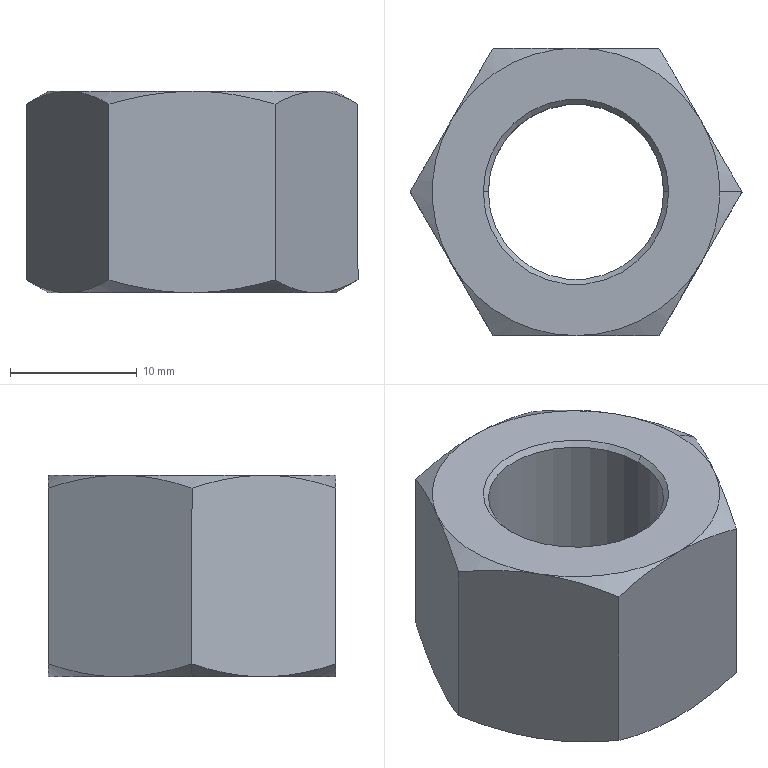Part | SolidWorks | features Cut 2, Chamfer 1, Extrusion 1 | 1 solid | 28 faces | box 26.2 x 22.69 x 15.9 mm | volume 4666 mm3 | cone 18 | plane 8 | cylinder 2 | commonest cylinder face diameters 13.835 x2
STEP:
#1=CARTESIAN_POINT('',(-6.918,0.,15.503));
#2=VERTEX_POINT('',#1);
#3=CARTESIAN_POINT('',(6.918,0.,15.503));
#4=VERTEX_POINT('',#3);
#5=CARTESIAN_POINT('',(0.,0.,15.503));
#6=DIRECTION('',(0.,0.,1.));
#7=DIRECTION('',(-1.,0.,0.));
#8=AXIS2_PLACEMENT_3D('',#5,#6,#7);
#9=CIRCLE('',#8,6.918);
#10=EDGE_CURVE('',#2,#4,#9,.T.);
#11=ORIENTED_EDGE('',*,*,#10,.F.);
#12=CARTESIAN_POINT('',(-7.315,0.,15.9));
#13=VERTEX_POINT('',#12);
#14=CARTESIAN_POINT('',(-6.918,0.,15.503));
#15=DIRECTION('',(-0.7071,0.,0.7071));
#16=VECTOR('',#15,1000.);
#17=LINE('',#14,#16);
#18=EDGE_CURVE('',#2,#13,#17,.T.);
#19=ORIENTED_EDGE('',*,*,#18,.T.);
#20=CARTESIAN_POINT('',(7.315,0.,15.9));
#21=VERTEX_POINT('',#20);
#22=CARTESIAN_POINT('',(0.,0.,15.9));
#23=DIRECTION('',(0.,0.,-1.));
#24=DIRECTION('',(-1.,0.,0.));
#25=AXIS2_PLACEMENT_3D('',#22,#23,#24);
#26=CIRCLE('',#25,7.315);
#27=EDGE_CURVE('',#21,#13,#26,.T.);
#28=ORIENTED_EDGE('',*,*,#27,.F.);
#29=CARTESIAN_POINT('',(6.918,0.,15.503));
#30=DIRECTION('',(0.7071,0.,0.7071));
#31=VECTOR('',#30,1000.);
#32=LINE('',#29,#31);
#33=EDGE_CURVE('',#4,#21,#32,.T.);
#34=ORIENTED_EDGE('',*,*,#33,.F.);
#35=EDGE_LOOP('',(#11,#19,#28,#34));
#36=FACE_OUTER_BOUND('',#35,.T.);
#37=CARTESIAN_POINT('',(0.,0.,15.503));
#38=DIRECTION('',(0.,0.,1.));
#39=DIRECTION('',(1.,0.,0.));
#40=AXIS2_PLACEMENT_3D('',#37,#38,#39);
#41=CONICAL_SURFACE('',#40,6.918,0.7854);
#42=ADVANCED_FACE('',(#36),#41,.F.);
#43=CARTESIAN_POINT('',(6.918,0.,0.3975));
#44=VERTEX_POINT('',#43);
#45=CARTESIAN_POINT('',(-6.918,0.,0.3975));
#46=VERTEX_POINT('',#45);
#47=CARTESIAN_POINT('',(0.,0.,0.3975));
#48=DIRECTION('',(0.,0.,-1.));
#49=DIRECTION('',(-1.,0.,0.));
#50=AXIS2_PLACEMENT_3D('',#47,#48,#49);
#51=CIRCLE('',#50,6.918);
#52=EDGE_CURVE('',#44,#46,#51,.T.);
#53=ORIENTED_EDGE('',*,*,#52,.F.);
#54=CARTESIAN_POINT('',(7.315,0.,0.));
#55=VERTEX_POINT('',#54);
#56=CARTESIAN_POINT('',(7.315,0.,0.));
#57=DIRECTION('',(0.7071,0.,-0.7071));
#58=VECTOR('',#57,1000.);
#59=LINE('',#56,#58);
#60=EDGE_CURVE('',#44,#55,#59,.T.);
#61=ORIENTED_EDGE('',*,*,#60,.T.);
#62=CARTESIAN_POINT('',(-7.315,0.,0.));
#63=VERTEX_POINT('',#62);
#64=CARTESIAN_POINT('',(0.,0.,0.));
#65=DIRECTION('',(0.,0.,1.));
#66=DIRECTION('',(-1.,0.,0.));
#67=AXIS2_PLACEMENT_3D('',#64,#65,#66);
#68=CIRCLE('',#67,7.315);
#69=EDGE_CURVE('',#63,#55,#68,.T.);
#70=ORIENTED_EDGE('',*,*,#69,.F.);
#71=CARTESIAN_POINT('',(-7.315,0.,0.));
#72=DIRECTION('',(-0.7071,0.,-0.7071));
#73=VECTOR('',#72,1000.);
#74=LINE('',#71,#73);
#75=EDGE_CURVE('',#46,#63,#74,.T.);
#76=ORIENTED_EDGE('',*,*,#75,.F.);
#77=EDGE_LOOP('',(#53,#61,#70,#76));
#78=FACE_OUTER_BOUND('',#77,.T.);
#79=CARTESIAN_POINT('',(0.,0.,0.));
#80=DIRECTION('',(0.,0.,-1.));
#81=DIRECTION('',(-1.,0.,0.));
#82=AXIS2_PLACEMENT_3D('',#79,#80,#81);
#83=CONICAL_SURFACE('',#82,7.315,0.7854);
#84=ADVANCED_FACE('',(#78),#83,.F.);
#85=CARTESIAN_POINT('',(9.825,5.672,15.9));
#86=VERTEX_POINT('',#85);
#87=CARTESIAN_POINT('',(11.345,0.,15.9));
#88=VERTEX_POINT('',#87);
#89=CARTESIAN_POINT('',(0.,0.,15.9));
#90=DIRECTION('',(0.,0.,-1.));
#91=DIRECTION('',(-1.,0.,0.));
#92=AXIS2_PLACEMENT_3D('',#89,#90,#91);
#93=CIRCLE('',#92,11.345);
#94=EDGE_CURVE('',#86,#88,#93,.T.);
#95=ORIENTED_EDGE('',*,*,#94,.T.);
#96=CARTESIAN_POINT('',(13.1,0.,14.887));
#97=VERTEX_POINT('',#96);
#98=CARTESIAN_POINT('',(11.345,0.,15.9));
#99=DIRECTION('',(0.866,0.,-0.5));
#100=VECTOR('',#99,1000.);
#101=LINE('',#98,#100);
#102=EDGE_CURVE('',#88,#97,#101,.T.);
#103=ORIENTED_EDGE('',*,*,#102,.T.);
#104=CARTESIAN_POINT('',(13.1,0.,14.887));
#105=CARTESIAN_POINT('',(12.564,0.9279,15.196));
#106=CARTESIAN_POINT('',(12.025,1.863,15.451));
#107=CARTESIAN_POINT('',(10.934,3.752,15.803));
#108=CARTESIAN_POINT('',(10.383,4.706,15.9));
#109=CARTESIAN_POINT('',(9.825,5.672,15.9));
#110=B_SPLINE_CURVE_WITH_KNOTS('',3,(#104,#105,#106,#107,#108,#109),.UNSPECIFIED.,.F.,.F.,(4,2,4),(0.000000238,0.003314,0.006628),.UNSPECIFIED.);
#111=EDGE_CURVE('',#97,#86,#110,.T.);
#112=ORIENTED_EDGE('',*,*,#111,.T.);
#113=EDGE_LOOP('',(#95,#103,#112));
#114=FACE_OUTER_BOUND('',#113,.T.);
#115=CARTESIAN_POINT('',(0.,0.,15.9));
#116=DIRECTION('',(0.,0.,-1.));
#117=DIRECTION('',(1.,0.,0.));
#118=AXIS2_PLACEMENT_3D('',#115,#116,#117);
#119=CONICAL_SURFACE('',#118,11.345,1.047);
#120=ADVANCED_FACE('',(#114),#119,.T.);
#121=CARTESIAN_POINT('',(-11.345,0.,0.));
#122=VERTEX_POINT('',#121);
#123=CARTESIAN_POINT('',(-9.825,5.672,0.));
#124=VERTEX_POINT('',#123);
#125=CARTESIAN_POINT('',(0.,0.,0.));
#126=DIRECTION('',(0.,0.,-1.));
#127=DIRECTION('',(-1.,0.,0.));
#128=AXIS2_PLACEMENT_3D('',#125,#126,#127);
#129=CIRCLE('',#128,11.345);
#130=EDGE_CURVE('',#122,#124,#129,.T.);
#131=ORIENTED_EDGE('',*,*,#130,.F.);
#132=CARTESIAN_POINT('',(-13.1,0.,1.013));
#133=VERTEX_POINT('',#132);
#134=CARTESIAN_POINT('',(-11.345,0.,0.));
#135=DIRECTION('',(-0.866,0.,0.5));
#136=VECTOR('',#135,1000.);
#137=LINE('',#134,#136);
#138=EDGE_CURVE('',#122,#133,#137,.T.);
#139=ORIENTED_EDGE('',*,*,#138,.T.);
#140=CARTESIAN_POINT('',(-13.1,0.,1.013));
#141=CARTESIAN_POINT('',(-12.564,0.9279,0.704));
#142=CARTESIAN_POINT('',(-12.025,1.863,0.4491));
#143=CARTESIAN_POINT('',(-10.934,3.752,0.09657));
#144=CARTESIAN_POINT('',(-10.383,4.706,0.));
#145=CARTESIAN_POINT('',(-9.825,5.672,0.));
#146=B_SPLINE_CURVE_WITH_KNOTS('',3,(#140,#141,#142,#143,#144,#145),.UNSPECIFIED.,.F.,.F.,(4,2,4),(0.000000238,0.003314,0.006628),.UNSPECIFIED.);
#147=EDGE_CURVE('',#133,#124,#146,.T.);
#148=ORIENTED_EDGE('',*,*,#147,.T.);
#149=EDGE_LOOP('',(#131,#139,#148));
#150=FACE_OUTER_BOUND('',#149,.T.);
#151=CARTESIAN_POINT('',(0.,0.,0.));
#152=DIRECTION('',(0.,0.,1.));
#153=DIRECTION('',(-1.,0.,0.));
#154=AXIS2_PLACEMENT_3D('',#151,#152,#153);
#155=CONICAL_SURFACE('',#154,11.345,1.047);
#156=ADVANCED_FACE('',(#150),#155,.T.);
#157=ORIENTED_EDGE('',*,*,#10,.T.);
#158=CARTESIAN_POINT('',(6.918,0.,15.9));
#159=DIRECTION('',(0.,0.,-1.));
#160=VECTOR('',#159,1000.);
#161=LINE('',#158,#160);
#162=EDGE_CURVE('',#4,#44,#161,.T.);
#163=ORIENTED_EDGE('',*,*,#162,.T.);
#164=ORIENTED_EDGE('',*,*,#52,.T.);
#165=CARTESIAN_POINT('',(-6.918,0.,15.9));
#166=DIRECTION('',(0.,0.,-1.));
#167=VECTOR('',#166,1000.);
#168=LINE('',#165,#167);
#169=EDGE_CURVE('',#2,#46,#168,.T.);
#170=ORIENTED_EDGE('',*,*,#169,.F.);
#171=EDGE_LOOP('',(#157,#163,#164,#170));
#172=FACE_OUTER_BOUND('',#171,.T.);
#173=CARTESIAN_POINT('',(0.,0.,15.9));
#174=DIRECTION('',(0.,0.,-1.));
#175=DIRECTION('',(-1.,0.,0.));
#176=AXIS2_PLACEMENT_3D('',#173,#174,#175);
#177=CYLINDRICAL_SURFACE('',#176,6.918);
#178=ADVANCED_FACE('',(#172),#177,.F.);
#179=ORIENTED_EDGE('',*,*,#111,.F.);
#180=CARTESIAN_POINT('',(13.1,0.,1.013));
#181=VERTEX_POINT('',#180);
#182=CARTESIAN_POINT('',(13.1,0.,15.9));
#183=DIRECTION('',(0.,0.,-1.));
#184=VECTOR('',#183,1000.);
#185=LINE('',#182,#184);
#186=EDGE_CURVE('',#97,#181,#185,.T.);
#187=ORIENTED_EDGE('',*,*,#186,.T.);
#188=CARTESIAN_POINT('',(9.825,5.672,0.));
#189=VERTEX_POINT('',#188);
#190=CARTESIAN_POINT('',(9.825,5.672,0.));
#191=CARTESIAN_POINT('',(10.103,5.191,0.));
#192=CARTESIAN_POINT('',(10.382,4.707,0.02395));
#193=CARTESIAN_POINT('',(10.934,3.751,0.1166));
#194=CARTESIAN_POINT('',(11.209,3.276,0.1853));
#195=CARTESIAN_POINT('',(12.027,1.859,0.45));
#196=CARTESIAN_POINT('',(12.566,0.9256,0.7047));
#197=CARTESIAN_POINT('',(13.1,0.,1.013));
#198=B_SPLINE_CURVE_WITH_KNOTS('',3,(#190,#191,#192,#193,#194,#195,#196,#197),.UNSPECIFIED.,.F.,.F.,(4,2,2,4),(0.006628,0.008278,0.009929,0.01323),.UNSPECIFIED.);
#199=EDGE_CURVE('',#189,#181,#198,.T.);
#200=ORIENTED_EDGE('',*,*,#199,.F.);
#201=CARTESIAN_POINT('',(6.55,11.345,1.013));
#202=VERTEX_POINT('',#201);
#203=CARTESIAN_POINT('',(6.55,11.345,1.013));
#204=CARTESIAN_POINT('',(7.086,10.417,0.704));
#205=CARTESIAN_POINT('',(7.625,9.482,0.4491));
#206=CARTESIAN_POINT('',(8.716,7.593,0.09657));
#207=CARTESIAN_POINT('',(9.267,6.639,0.));
#208=CARTESIAN_POINT('',(9.825,5.672,0.));
#209=B_SPLINE_CURVE_WITH_KNOTS('',3,(#203,#204,#205,#206,#207,#208),.UNSPECIFIED.,.F.,.F.,(4,2,4),(0.000000238,0.003314,0.006628),.UNSPECIFIED.);
#210=EDGE_CURVE('',#202,#189,#209,.T.);
#211=ORIENTED_EDGE('',*,*,#210,.F.);
#212=CARTESIAN_POINT('',(6.55,11.345,14.887));
#213=VERTEX_POINT('',#212);
#214=CARTESIAN_POINT('',(6.55,11.345,15.9));
#215=DIRECTION('',(0.,0.,-1.));
#216=VECTOR('',#215,1000.);
#217=LINE('',#214,#216);
#218=EDGE_CURVE('',#213,#202,#217,.T.);
#219=ORIENTED_EDGE('',*,*,#218,.F.);
#220=CARTESIAN_POINT('',(9.825,5.672,15.9));
#221=CARTESIAN_POINT('',(9.547,6.154,15.9));
#222=CARTESIAN_POINT('',(9.268,6.637,15.876));
#223=CARTESIAN_POINT('',(8.716,7.594,15.783));
#224=CARTESIAN_POINT('',(8.441,8.069,15.715));
#225=CARTESIAN_POINT('',(7.623,9.486,15.45));
#226=CARTESIAN_POINT('',(7.084,10.419,15.195));
#227=CARTESIAN_POINT('',(6.55,11.345,14.887));
#228=B_SPLINE_CURVE_WITH_KNOTS('',3,(#220,#221,#222,#223,#224,#225,#226,#227),.UNSPECIFIED.,.F.,.F.,(4,2,2,4),(0.006628,0.008278,0.009929,0.01323),.UNSPECIFIED.);
#229=EDGE_CURVE('',#86,#213,#228,.T.);
#230=ORIENTED_EDGE('',*,*,#229,.F.);
#231=EDGE_LOOP('',(#179,#187,#200,#211,#219,#230));
#232=FACE_OUTER_BOUND('',#231,.T.);
#233=CARTESIAN_POINT('',(13.1,0.,15.9));
#234=DIRECTION('',(-0.866,-0.5,0.));
#235=DIRECTION('',(0.5,-0.866,0.));
#236=AXIS2_PLACEMENT_3D('',#233,#234,#235);
#237=PLANE('',#236);
#238=ADVANCED_FACE('',(#232),#237,.F.);
#239=CARTESIAN_POINT('',(0.,11.345,15.9));
#240=VERTEX_POINT('',#239);
#241=CARTESIAN_POINT('',(6.55,11.345,14.887));
#242=CARTESIAN_POINT('',(5.491,11.345,15.193));
#243=CARTESIAN_POINT('',(4.418,11.345,15.447));
#244=CARTESIAN_POINT('',(2.778,11.345,15.713));
#245=CARTESIAN_POINT('',(2.227,11.345,15.783));
#246=CARTESIAN_POINT('',(1.112,11.345,15.876));
#247=CARTESIAN_POINT('',(0.5544,11.345,15.9));
#248=CARTESIAN_POINT('',(0.,11.345,15.9));
#249=B_SPLINE_CURVE_WITH_KNOTS('',3,(#241,#242,#243,#244,#245,#246,#247,#248),.UNSPECIFIED.,.F.,.F.,(4,2,2,4),(0.03911,0.04243,0.04409,0.04574),.UNSPECIFIED.);
#250=EDGE_CURVE('',#213,#240,#249,.T.);
#251=ORIENTED_EDGE('',*,*,#250,.F.);
#252=ORIENTED_EDGE('',*,*,#218,.T.);
#253=CARTESIAN_POINT('',(0.,11.345,0.));
#254=VERTEX_POINT('',#253);
#255=CARTESIAN_POINT('',(0.,11.345,0.));
#256=CARTESIAN_POINT('',(0.5544,11.345,0.));
#257=CARTESIAN_POINT('',(1.112,11.345,0.02366));
#258=CARTESIAN_POINT('',(2.227,11.345,0.1174));
#259=CARTESIAN_POINT('',(2.778,11.345,0.1867));
#260=CARTESIAN_POINT('',(4.418,11.345,0.453));
#261=CARTESIAN_POINT('',(5.491,11.345,0.7075));
#262=CARTESIAN_POINT('',(6.55,11.345,1.013));
#263=B_SPLINE_CURVE_WITH_KNOTS('',3,(#255,#256,#257,#258,#259,#260,#261,#262),.UNSPECIFIED.,.F.,.F.,(4,2,2,4),(0.01869,0.02035,0.02201,0.02533),.UNSPECIFIED.);
#264=EDGE_CURVE('',#254,#202,#263,.T.);
#265=ORIENTED_EDGE('',*,*,#264,.F.);
#266=CARTESIAN_POINT('',(-6.55,11.345,1.013));
#267=VERTEX_POINT('',#266);
#268=CARTESIAN_POINT('',(-6.55,11.345,1.013));
#269=CARTESIAN_POINT('',(-5.484,11.345,0.7054));
#270=CARTESIAN_POINT('',(-4.393,11.345,0.4478));
#271=CARTESIAN_POINT('',(-2.208,11.345,0.09531));
#272=CARTESIAN_POINT('',(-1.108,11.345,0.));
#273=CARTESIAN_POINT('',(0.,11.345,0.));
#274=B_SPLINE_CURVE_WITH_KNOTS('',3,(#268,#269,#270,#271,#272,#273),.UNSPECIFIED.,.F.,.F.,(4,2,4),(0.01206,0.01538,0.01869),.UNSPECIFIED.);
#275=EDGE_CURVE('',#267,#254,#274,.T.);
#276=ORIENTED_EDGE('',*,*,#275,.F.);
#277=CARTESIAN_POINT('',(-6.55,11.345,14.887));
#278=VERTEX_POINT('',#277);
#279=CARTESIAN_POINT('',(-6.55,11.345,15.9));
#280=DIRECTION('',(0.,0.,-1.));
#281=VECTOR('',#280,1000.);
#282=LINE('',#279,#281);
#283=EDGE_CURVE('',#278,#267,#282,.T.);
#284=ORIENTED_EDGE('',*,*,#283,.F.);
#285=CARTESIAN_POINT('',(0.,11.345,15.9));
#286=CARTESIAN_POINT('',(-1.108,11.345,15.9));
#287=CARTESIAN_POINT('',(-2.208,11.345,15.805));
#288=CARTESIAN_POINT('',(-4.393,11.345,15.452));
#289=CARTESIAN_POINT('',(-5.484,11.345,15.195));
#290=CARTESIAN_POINT('',(-6.55,11.345,14.887));
#291=B_SPLINE_CURVE_WITH_KNOTS('',3,(#285,#286,#287,#288,#289,#290),.UNSPECIFIED.,.F.,.F.,(4,2,4),(0.04574,0.04906,0.05237),.UNSPECIFIED.);
#292=EDGE_CURVE('',#240,#278,#291,.T.);
#293=ORIENTED_EDGE('',*,*,#292,.F.);
#294=EDGE_LOOP('',(#251,#252,#265,#276,#284,#293));
#295=FACE_OUTER_BOUND('',#294,.T.);
#296=CARTESIAN_POINT('',(6.55,11.345,15.9));
#297=DIRECTION('',(0.,-1.,0.));
#298=DIRECTION('',(1.,0.,0.));
#299=AXIS2_PLACEMENT_3D('',#296,#297,#298);
#300=PLANE('',#299);
#301=ADVANCED_FACE('',(#295),#300,.F.);
#302=CARTESIAN_POINT('',(-9.825,5.672,15.9));
#303=VERTEX_POINT('',#302);
#304=CARTESIAN_POINT('',(-6.55,11.345,14.887));
#305=CARTESIAN_POINT('',(-7.086,10.417,15.196));
#306=CARTESIAN_POINT('',(-7.625,9.482,15.451));
#307=CARTESIAN_POINT('',(-8.716,7.593,15.803));
#308=CARTESIAN_POINT('',(-9.267,6.639,15.9));
#309=CARTESIAN_POINT('',(-9.825,5.672,15.9));
#310=B_SPLINE_CURVE_WITH_KNOTS('',3,(#304,#305,#306,#307,#308,#309),.UNSPECIFIED.,.F.,.F.,(4,2,4),(0.000000238,0.003314,0.006628),.UNSPECIFIED.);
#311=EDGE_CURVE('',#278,#303,#310,.T.);
#312=ORIENTED_EDGE('',*,*,#311,.F.);
#313=ORIENTED_EDGE('',*,*,#283,.T.);
#314=CARTESIAN_POINT('',(-9.825,5.672,0.));
#315=CARTESIAN_POINT('',(-9.547,6.154,0.));
#316=CARTESIAN_POINT('',(-9.268,6.637,0.02395));
#317=CARTESIAN_POINT('',(-8.716,7.594,0.1166));
#318=CARTESIAN_POINT('',(-8.441,8.069,0.1853));
#319=CARTESIAN_POINT('',(-7.623,9.486,0.45));
#320=CARTESIAN_POINT('',(-7.084,10.419,0.7047));
#321=CARTESIAN_POINT('',(-6.55,11.345,1.013));
#322=B_SPLINE_CURVE_WITH_KNOTS('',3,(#314,#315,#316,#317,#318,#319,#320,#321),.UNSPECIFIED.,.F.,.F.,(4,2,2,4),(0.006628,0.008278,0.009929,0.01323),.UNSPECIFIED.);
#323=EDGE_CURVE('',#124,#267,#322,.T.);
#324=ORIENTED_EDGE('',*,*,#323,.F.);
#325=ORIENTED_EDGE('',*,*,#147,.F.);
#326=CARTESIAN_POINT('',(-13.1,0.,14.887));
#327=VERTEX_POINT('',#326);
#328=CARTESIAN_POINT('',(-13.1,0.,15.9));
#329=DIRECTION('',(0.,0.,-1.));
#330=VECTOR('',#329,1000.);
#331=LINE('',#328,#330);
#332=EDGE_CURVE('',#327,#133,#331,.T.);
#333=ORIENTED_EDGE('',*,*,#332,.F.);
#334=CARTESIAN_POINT('',(-9.825,5.672,15.9));
#335=CARTESIAN_POINT('',(-10.103,5.191,15.9));
#336=CARTESIAN_POINT('',(-10.382,4.707,15.876));
#337=CARTESIAN_POINT('',(-10.934,3.751,15.783));
#338=CARTESIAN_POINT('',(-11.209,3.276,15.715));
#339=CARTESIAN_POINT('',(-12.027,1.859,15.45));
#340=CARTESIAN_POINT('',(-12.566,0.9256,15.195));
#341=CARTESIAN_POINT('',(-13.1,0.,14.887));
#342=B_SPLINE_CURVE_WITH_KNOTS('',3,(#334,#335,#336,#337,#338,#339,#340,#341),.UNSPECIFIED.,.F.,.F.,(4,2,2,4),(0.006628,0.008278,0.009929,0.01323),.UNSPECIFIED.);
#343=EDGE_CURVE('',#303,#327,#342,.T.);
#344=ORIENTED_EDGE('',*,*,#343,.F.);
#345=EDGE_LOOP('',(#312,#313,#324,#325,#333,#344));
#346=FACE_OUTER_BOUND('',#345,.T.);
#347=CARTESIAN_POINT('',(-6.55,11.345,15.9));
#348=DIRECTION('',(0.866,-0.5,0.));
#349=DIRECTION('',(0.5,0.866,0.));
#350=AXIS2_PLACEMENT_3D('',#347,#348,#349);
#351=PLANE('',#350);
#352=ADVANCED_FACE('',(#346),#351,.F.);
#353=CARTESIAN_POINT('',(-9.825,-5.672,15.9));
#354=VERTEX_POINT('',#353);
#355=CARTESIAN_POINT('',(-13.1,0.,14.887));
#356=CARTESIAN_POINT('',(-12.564,-0.9279,15.196));
#357=CARTESIAN_POINT('',(-12.025,-1.863,15.451));
#358=CARTESIAN_POINT('',(-10.934,-3.752,15.803));
#359=CARTESIAN_POINT('',(-10.383,-4.706,15.9));
#360=CARTESIAN_POINT('',(-9.825,-5.672,15.9));
#361=B_SPLINE_CURVE_WITH_KNOTS('',3,(#355,#356,#357,#358,#359,#360),.UNSPECIFIED.,.F.,.F.,(4,2,4),(0.000000238,0.003314,0.006628),.UNSPECIFIED.);
#362=EDGE_CURVE('',#327,#354,#361,.T.);
#363=ORIENTED_EDGE('',*,*,#362,.F.);
#364=ORIENTED_EDGE('',*,*,#332,.T.);
#365=CARTESIAN_POINT('',(-9.825,-5.672,0.));
#366=VERTEX_POINT('',#365);
#367=CARTESIAN_POINT('',(-9.825,-5.672,0.));
#368=CARTESIAN_POINT('',(-10.103,-5.191,0.));
#369=CARTESIAN_POINT('',(-10.382,-4.707,0.02395));
#370=CARTESIAN_POINT('',(-10.934,-3.751,0.1166));
#371=CARTESIAN_POINT('',(-11.209,-3.276,0.1853));
#372=CARTESIAN_POINT('',(-12.027,-1.859,0.45));
#373=CARTESIAN_POINT('',(-12.566,-0.9256,0.7047));
#374=CARTESIAN_POINT('',(-13.1,0.,1.013));
#375=B_SPLINE_CURVE_WITH_KNOTS('',3,(#367,#368,#369,#370,#371,#372,#373,#374),.UNSPECIFIED.,.F.,.F.,(4,2,2,4),(0.006628,0.008278,0.009929,0.01323),.UNSPECIFIED.);
#376=EDGE_CURVE('',#366,#133,#375,.T.);
#377=ORIENTED_EDGE('',*,*,#376,.F.);
#378=CARTESIAN_POINT('',(-6.55,-11.345,1.013));
#379=VERTEX_POINT('',#378);
#380=CARTESIAN_POINT('',(-6.55,-11.345,1.013));
#381=CARTESIAN_POINT('',(-7.086,-10.417,0.704));
#382=CARTESIAN_POINT('',(-7.625,-9.482,0.4491));
#383=CARTESIAN_POINT('',(-8.716,-7.593,0.09657));
#384=CARTESIAN_POINT('',(-9.267,-6.639,0.));
#385=CARTESIAN_POINT('',(-9.825,-5.672,0.));
#386=B_SPLINE_CURVE_WITH_KNOTS('',3,(#380,#381,#382,#383,#384,#385),.UNSPECIFIED.,.F.,.F.,(4,2,4),(0.000000238,0.003314,0.006628),.UNSPECIFIED.);
#387=EDGE_CURVE('',#379,#366,#386,.T.);
#388=ORIENTED_EDGE('',*,*,#387,.F.);
#389=CARTESIAN_POINT('',(-6.55,-11.345,14.887));
#390=VERTEX_POINT('',#389);
#391=CARTESIAN_POINT('',(-6.55,-11.345,15.9));
#392=DIRECTION('',(0.,0.,-1.));
#393=VECTOR('',#392,1000.);
#394=LINE('',#391,#393);
#395=EDGE_CURVE('',#390,#379,#394,.T.);
#396=ORIENTED_EDGE('',*,*,#395,.F.);
#397=CARTESIAN_POINT('',(-9.825,-5.672,15.9));
#398=CARTESIAN_POINT('',(-9.547,-6.154,15.9));
#399=CARTESIAN_POINT('',(-9.268,-6.637,15.876));
#400=CARTESIAN_POINT('',(-8.716,-7.594,15.783));
#401=CARTESIAN_POINT('',(-8.441,-8.069,15.715));
#402=CARTESIAN_POINT('',(-7.623,-9.486,15.45));
#403=CARTESIAN_POINT('',(-7.084,-10.419,15.195));
#404=CARTESIAN_POINT('',(-6.55,-11.345,14.887));
#405=B_SPLINE_CURVE_WITH_KNOTS('',3,(#397,#398,#399,#400,#401,#402,#403,#404),.UNSPECIFIED.,.F.,.F.,(4,2,2,4),(0.006628,0.008278,0.009929,0.01323),.UNSPECIFIED.);
#406=EDGE_CURVE('',#354,#390,#405,.T.);
#407=ORIENTED_EDGE('',*,*,#406,.F.);
#408=EDGE_LOOP('',(#363,#364,#377,#388,#396,#407));
#409=FACE_OUTER_BOUND('',#408,.T.);
#410=CARTESIAN_POINT('',(-13.1,0.,15.9));
#411=DIRECTION('',(0.866,0.5,0.));
#412=DIRECTION('',(-0.5,0.866,0.));
#413=AXIS2_PLACEMENT_3D('',#410,#411,#412);
#414=PLANE('',#413);
#415=ADVANCED_FACE('',(#409),#414,.F.);
#416=CARTESIAN_POINT('',(0.,-11.345,15.9));
#417=VERTEX_POINT('',#416);
#418=CARTESIAN_POINT('',(-6.55,-11.345,14.887));
#419=CARTESIAN_POINT('',(-5.484,-11.345,15.195));
#420=CARTESIAN_POINT('',(-4.393,-11.345,15.452));
#421=CARTESIAN_POINT('',(-2.208,-11.345,15.805));
#422=CARTESIAN_POINT('',(-1.108,-11.345,15.9));
#423=CARTESIAN_POINT('',(0.,-11.345,15.9));
#424=B_SPLINE_CURVE_WITH_KNOTS('',3,(#418,#419,#420,#421,#422,#423),.UNSPECIFIED.,.F.,.F.,(4,2,4),(0.01206,0.01538,0.01869),.UNSPECIFIED.);
#425=EDGE_CURVE('',#390,#417,#424,.T.);
#426=ORIENTED_EDGE('',*,*,#425,.F.);
#427=ORIENTED_EDGE('',*,*,#395,.T.);
#428=CARTESIAN_POINT('',(0.,-11.345,0.));
#429=VERTEX_POINT('',#428);
#430=CARTESIAN_POINT('',(0.,-11.345,0.));
#431=CARTESIAN_POINT('',(-1.108,-11.345,0.));
#432=CARTESIAN_POINT('',(-2.208,-11.345,0.09531));
#433=CARTESIAN_POINT('',(-4.393,-11.345,0.4478));
#434=CARTESIAN_POINT('',(-5.484,-11.345,0.7054));
#435=CARTESIAN_POINT('',(-6.55,-11.345,1.013));
#436=B_SPLINE_CURVE_WITH_KNOTS('',3,(#430,#431,#432,#433,#434,#435),.UNSPECIFIED.,.F.,.F.,(4,2,4),(0.04574,0.04906,0.05237),.UNSPECIFIED.);
#437=EDGE_CURVE('',#429,#379,#436,.T.);
#438=ORIENTED_EDGE('',*,*,#437,.F.);
#439=CARTESIAN_POINT('',(6.55,-11.345,1.013));
#440=VERTEX_POINT('',#439);
#441=CARTESIAN_POINT('',(6.55,-11.345,1.013));
#442=CARTESIAN_POINT('',(5.491,-11.345,0.7075));
#443=CARTESIAN_POINT('',(4.418,-11.345,0.453));
#444=CARTESIAN_POINT('',(2.778,-11.345,0.1867));
#445=CARTESIAN_POINT('',(2.227,-11.345,0.1174));
#446=CARTESIAN_POINT('',(1.112,-11.345,0.02366));
#447=CARTESIAN_POINT('',(0.5544,-11.345,0.));
#448=CARTESIAN_POINT('',(0.,-11.345,0.));
#449=B_SPLINE_CURVE_WITH_KNOTS('',3,(#441,#442,#443,#444,#445,#446,#447,#448),.UNSPECIFIED.,.F.,.F.,(4,2,2,4),(0.03911,0.04243,0.04409,0.04574),.UNSPECIFIED.);
#450=EDGE_CURVE('',#440,#429,#449,.T.);
#451=ORIENTED_EDGE('',*,*,#450,.F.);
#452=CARTESIAN_POINT('',(6.55,-11.345,14.887));
#453=VERTEX_POINT('',#452);
#454=CARTESIAN_POINT('',(6.55,-11.345,15.9));
#455=DIRECTION('',(0.,0.,-1.));
#456=VECTOR('',#455,1000.);
#457=LINE('',#454,#456);
#458=EDGE_CURVE('',#453,#440,#457,.T.);
#459=ORIENTED_EDGE('',*,*,#458,.F.);
#460=CARTESIAN_POINT('',(0.,-11.345,15.9));
#461=CARTESIAN_POINT('',(0.5544,-11.345,15.9));
#462=CARTESIAN_POINT('',(1.112,-11.345,15.876));
#463=CARTESIAN_POINT('',(2.227,-11.345,15.783));
#464=CARTESIAN_POINT('',(2.778,-11.345,15.713));
#465=CARTESIAN_POINT('',(4.418,-11.345,15.447));
#466=CARTESIAN_POINT('',(5.491,-11.345,15.193));
#467=CARTESIAN_POINT('',(6.55,-11.345,14.887));
#468=B_SPLINE_CURVE_WITH_KNOTS('',3,(#460,#461,#462,#463,#464,#465,#466,#467),.UNSPECIFIED.,.F.,.F.,(4,2,2,4),(0.01869,0.02035,0.02201,0.02533),.UNSPECIFIED.);
#469=EDGE_CURVE('',#417,#453,#468,.T.);
#470=ORIENTED_EDGE('',*,*,#469,.F.);
#471=EDGE_LOOP('',(#426,#427,#438,#451,#459,#470));
#472=FACE_OUTER_BOUND('',#471,.T.);
#473=CARTESIAN_POINT('',(-6.55,-11.345,15.9));
#474=DIRECTION('',(0.,1.,0.));
#475=DIRECTION('',(-1.,0.,0.));
#476=AXIS2_PLACEMENT_3D('',#473,#474,#475);
#477=PLANE('',#476);
#478=ADVANCED_FACE('',(#472),#477,.F.);
#479=CARTESIAN_POINT('',(9.825,-5.672,15.9));
#480=VERTEX_POINT('',#479);
#481=CARTESIAN_POINT('',(6.55,-11.345,14.887));
#482=CARTESIAN_POINT('',(7.086,-10.417,15.196));
#483=CARTESIAN_POINT('',(7.625,-9.482,15.451));
#484=CARTESIAN_POINT('',(8.716,-7.593,15.803));
#485=CARTESIAN_POINT('',(9.267,-6.639,15.9));
#486=CARTESIAN_POINT('',(9.825,-5.672,15.9));
#487=B_SPLINE_CURVE_WITH_KNOTS('',3,(#481,#482,#483,#484,#485,#486),.UNSPECIFIED.,.F.,.F.,(4,2,4),(0.000000238,0.003314,0.006628),.UNSPECIFIED.);
#488=EDGE_CURVE('',#453,#480,#487,.T.);
#489=ORIENTED_EDGE('',*,*,#488,.F.);
#490=ORIENTED_EDGE('',*,*,#458,.T.);
#491=CARTESIAN_POINT('',(9.825,-5.672,0.));
#492=VERTEX_POINT('',#491);
#493=CARTESIAN_POINT('',(9.825,-5.672,0.));
#494=CARTESIAN_POINT('',(9.547,-6.154,0.));
#495=CARTESIAN_POINT('',(9.268,-6.637,0.02395));
#496=CARTESIAN_POINT('',(8.716,-7.594,0.1166));
#497=CARTESIAN_POINT('',(8.441,-8.069,0.1853));
#498=CARTESIAN_POINT('',(7.623,-9.486,0.45));
#499=CARTESIAN_POINT('',(7.084,-10.419,0.7047));
#500=CARTESIAN_POINT('',(6.55,-11.345,1.013));
#501=B_SPLINE_CURVE_WITH_KNOTS('',3,(#493,#494,#495,#496,#497,#498,#499,#500),.UNSPECIFIED.,.F.,.F.,(4,2,2,4),(0.006628,0.008278,0.009929,0.01323),.UNSPECIFIED.);
#502=EDGE_CURVE('',#492,#440,#501,.T.);
#503=ORIENTED_EDGE('',*,*,#502,.F.);
#504=CARTESIAN_POINT('',(13.1,0.,1.013));
#505=CARTESIAN_POINT('',(12.564,-0.9279,0.704));
#506=CARTESIAN_POINT('',(12.025,-1.863,0.4491));
#507=CARTESIAN_POINT('',(10.934,-3.752,0.09657));
#508=CARTESIAN_POINT('',(10.383,-4.706,0.));
#509=CARTESIAN_POINT('',(9.825,-5.672,0.));
#510=B_SPLINE_CURVE_WITH_KNOTS('',3,(#504,#505,#506,#507,#508,#509),.UNSPECIFIED.,.F.,.F.,(4,2,4),(0.000000238,0.003314,0.006628),.UNSPECIFIED.);
#511=EDGE_CURVE('',#181,#492,#510,.T.);
#512=ORIENTED_EDGE('',*,*,#511,.F.);
#513=ORIENTED_EDGE('',*,*,#186,.F.);
#514=CARTESIAN_POINT('',(9.825,-5.672,15.9));
#515=CARTESIAN_POINT('',(10.103,-5.191,15.9));
#516=CARTESIAN_POINT('',(10.382,-4.707,15.876));
#517=CARTESIAN_POINT('',(10.934,-3.751,15.783));
#518=CARTESIAN_POINT('',(11.209,-3.276,15.715));
#519=CARTESIAN_POINT('',(12.027,-1.859,15.45));
#520=CARTESIAN_POINT('',(12.566,-0.9256,15.195));
#521=CARTESIAN_POINT('',(13.1,0.,14.887));
#522=B_SPLINE_CURVE_WITH_KNOTS('',3,(#514,#515,#516,#517,#518,#519,#520,#521),.UNSPECIFIED.,.F.,.F.,(4,2,2,4),(0.006628,0.008278,0.009929,0.01323),.UNSPECIFIED.);
#523=EDGE_CURVE('',#480,#97,#522,.T.);
#524=ORIENTED_EDGE('',*,*,#523,.F.);
#525=EDGE_LOOP('',(#489,#490,#503,#512,#513,#524));
#526=FACE_OUTER_BOUND('',#525,.T.);
#527=CARTESIAN_POINT('',(6.55,-11.345,15.9));
#528=DIRECTION('',(-0.866,0.5,0.));
#529=DIRECTION('',(-0.5,-0.866,0.));
#530=AXIS2_PLACEMENT_3D('',#527,#528,#529);
#531=PLANE('',#530);
#532=ADVANCED_FACE('',(#526),#531,.F.);
#533=ORIENTED_EDGE('',*,*,#27,.T.);
#534=CARTESIAN_POINT('',(0.,0.,15.9));
#535=DIRECTION('',(0.,0.,-1.));
#536=DIRECTION('',(-1.,0.,0.));
#537=AXIS2_PLACEMENT_3D('',#534,#535,#536);
#538=CIRCLE('',#537,7.315);
#539=EDGE_CURVE('',#13,#21,#538,.T.);
#540=ORIENTED_EDGE('',*,*,#539,.T.);
#541=EDGE_LOOP('',(#533,#540));
#542=FACE_BOUND('',#541,.T.);
#543=CARTESIAN_POINT('',(0.,0.,15.9));
#544=DIRECTION('',(0.,0.,-1.));
#545=DIRECTION('',(-1.,0.,0.));
#546=AXIS2_PLACEMENT_3D('',#543,#544,#545);
#547=CIRCLE('',#546,11.345);
#548=EDGE_CURVE('',#303,#240,#547,.T.);
#549=ORIENTED_EDGE('',*,*,#548,.F.);
#550=CARTESIAN_POINT('',(0.,0.,15.9));
#551=DIRECTION('',(0.,0.,-1.));
#552=DIRECTION('',(-1.,0.,0.));
#553=AXIS2_PLACEMENT_3D('',#550,#551,#552);
#554=CIRCLE('',#553,11.345);
#555=EDGE_CURVE('',#354,#303,#554,.T.);
#556=ORIENTED_EDGE('',*,*,#555,.F.);
#557=CARTESIAN_POINT('',(0.,0.,15.9));
#558=DIRECTION('',(0.,0.,-1.));
#559=DIRECTION('',(-1.,0.,0.));
#560=AXIS2_PLACEMENT_3D('',#557,#558,#559);
#561=CIRCLE('',#560,11.345);
#562=EDGE_CURVE('',#417,#354,#561,.T.);
#563=ORIENTED_EDGE('',*,*,#562,.F.);
#564=CARTESIAN_POINT('',(0.,0.,15.9));
#565=DIRECTION('',(0.,0.,-1.));
#566=DIRECTION('',(-1.,0.,0.));
#567=AXIS2_PLACEMENT_3D('',#564,#565,#566);
#568=CIRCLE('',#567,11.345);
#569=EDGE_CURVE('',#480,#417,#568,.T.);
#570=ORIENTED_EDGE('',*,*,#569,.F.);
#571=CARTESIAN_POINT('',(0.,0.,15.9));
#572=DIRECTION('',(0.,0.,-1.));
#573=DIRECTION('',(-1.,0.,0.));
#574=AXIS2_PLACEMENT_3D('',#571,#572,#573);
#575=CIRCLE('',#574,11.345);
#576=EDGE_CURVE('',#88,#480,#575,.T.);
#577=ORIENTED_EDGE('',*,*,#576,.F.);
#578=ORIENTED_EDGE('',*,*,#94,.F.);
#579=CARTESIAN_POINT('',(0.,0.,15.9));
#580=DIRECTION('',(0.,0.,1.));
#581=DIRECTION('',(1.,0.,0.));
#582=AXIS2_PLACEMENT_3D('',#579,#580,#581);
#583=CIRCLE('',#582,11.345);
#584=EDGE_CURVE('',#86,#240,#583,.T.);
#585=ORIENTED_EDGE('',*,*,#584,.T.);
#586=EDGE_LOOP('',(#549,#556,#563,#570,#577,#578,#585));
#587=FACE_OUTER_BOUND('',#586,.T.);
#588=CARTESIAN_POINT('',(13.1,0.,15.9));
#589=DIRECTION('',(0.,0.,-1.));
#590=DIRECTION('',(-1.,0.,0.));
#591=AXIS2_PLACEMENT_3D('',#588,#589,#590);
#592=PLANE('',#591);
#593=ADVANCED_FACE('',(#542,#587),#592,.F.);
#594=ORIENTED_EDGE('',*,*,#69,.T.);
#595=CARTESIAN_POINT('',(0.,0.,0.));
#596=DIRECTION('',(0.,0.,1.));
#597=DIRECTION('',(-1.,0.,0.));
#598=AXIS2_PLACEMENT_3D('',#595,#596,#597);
#599=CIRCLE('',#598,7.315);
#600=EDGE_CURVE('',#55,#63,#599,.T.);
#601=ORIENTED_EDGE('',*,*,#600,.T.);
#602=EDGE_LOOP('',(#594,#601));
#603=FACE_BOUND('',#602,.T.);
#604=CARTESIAN_POINT('',(0.,0.,0.));
#605=DIRECTION('',(0.,0.,-1.));
#606=DIRECTION('',(-1.,0.,0.));
#607=AXIS2_PLACEMENT_3D('',#604,#605,#606);
#608=CIRCLE('',#607,11.345);
#609=EDGE_CURVE('',#366,#122,#608,.T.);
#610=ORIENTED_EDGE('',*,*,#609,.T.);
#611=ORIENTED_EDGE('',*,*,#130,.T.);
#612=CARTESIAN_POINT('',(0.,0.,0.));
#613=DIRECTION('',(0.,0.,-1.));
#614=DIRECTION('',(-1.,0.,0.));
#615=AXIS2_PLACEMENT_3D('',#612,#613,#614);
#616=CIRCLE('',#615,11.345);
#617=EDGE_CURVE('',#124,#254,#616,.T.);
#618=ORIENTED_EDGE('',*,*,#617,.T.);
#619=CARTESIAN_POINT('',(0.,0.,0.));
#620=DIRECTION('',(0.,0.,-1.));
#621=DIRECTION('',(-1.,0.,0.));
#622=AXIS2_PLACEMENT_3D('',#619,#620,#621);
#623=CIRCLE('',#622,11.345);
#624=EDGE_CURVE('',#254,#189,#623,.T.);
#625=ORIENTED_EDGE('',*,*,#624,.T.);
#626=CARTESIAN_POINT('',(0.,0.,0.));
#627=DIRECTION('',(0.,0.,-1.));
#628=DIRECTION('',(-1.,0.,0.));
#629=AXIS2_PLACEMENT_3D('',#626,#627,#628);
#630=CIRCLE('',#629,11.345);
#631=EDGE_CURVE('',#189,#492,#630,.T.);
#632=ORIENTED_EDGE('',*,*,#631,.T.);
#633=CARTESIAN_POINT('',(0.,0.,0.));
#634=DIRECTION('',(0.,0.,-1.));
#635=DIRECTION('',(-1.,0.,0.));
#636=AXIS2_PLACEMENT_3D('',#633,#634,#635);
#637=CIRCLE('',#636,11.345);
#638=EDGE_CURVE('',#492,#429,#637,.T.);
#639=ORIENTED_EDGE('',*,*,#638,.T.);
#640=CARTESIAN_POINT('',(0.,0.,0.));
#641=DIRECTION('',(0.,0.,-1.));
#642=DIRECTION('',(-1.,0.,0.));
#643=AXIS2_PLACEMENT_3D('',#640,#641,#642);
#644=CIRCLE('',#643,11.345);
#645=EDGE_CURVE('',#429,#366,#644,.T.);
#646=ORIENTED_EDGE('',*,*,#645,.T.);
#647=EDGE_LOOP('',(#610,#611,#618,#625,#632,#639,#646));
#648=FACE_OUTER_BOUND('',#647,.T.);
#649=CARTESIAN_POINT('',(13.1,0.,0.));
#650=DIRECTION('',(0.,0.,-1.));
#651=DIRECTION('',(-1.,0.,0.));
#652=AXIS2_PLACEMENT_3D('',#649,#650,#651);
#653=PLANE('',#652);
#654=ADVANCED_FACE('',(#603,#648),#653,.T.);
#655=ORIENTED_EDGE('',*,*,#162,.F.);
#656=CARTESIAN_POINT('',(0.,0.,15.503));
#657=DIRECTION('',(0.,0.,1.));
#658=DIRECTION('',(-1.,0.,0.));
#659=AXIS2_PLACEMENT_3D('',#656,#657,#658);
#660=CIRCLE('',#659,6.918);
#661=EDGE_CURVE('',#4,#2,#660,.T.);
#662=ORIENTED_EDGE('',*,*,#661,.T.);
#663=ORIENTED_EDGE('',*,*,#169,.T.);
#664=CARTESIAN_POINT('',(0.,0.,0.3975));
#665=DIRECTION('',(0.,0.,-1.));
#666=DIRECTION('',(-1.,0.,0.));
#667=AXIS2_PLACEMENT_3D('',#664,#665,#666);
#668=CIRCLE('',#667,6.918);
#669=EDGE_CURVE('',#46,#44,#668,.T.);
#670=ORIENTED_EDGE('',*,*,#669,.T.);
#671=EDGE_LOOP('',(#655,#662,#663,#670));
#672=FACE_OUTER_BOUND('',#671,.T.);
#673=CARTESIAN_POINT('',(0.,0.,15.9));
#674=DIRECTION('',(0.,0.,-1.));
#675=DIRECTION('',(-1.,0.,0.));
#676=AXIS2_PLACEMENT_3D('',#673,#674,#675);
#677=CYLINDRICAL_SURFACE('',#676,6.918);
#678=ADVANCED_FACE('',(#672),#677,.F.);
#679=ORIENTED_EDGE('',*,*,#450,.T.);
#680=ORIENTED_EDGE('',*,*,#638,.F.);
#681=ORIENTED_EDGE('',*,*,#502,.T.);
#682=EDGE_LOOP('',(#679,#680,#681));
#683=FACE_OUTER_BOUND('',#682,.T.);
#684=CARTESIAN_POINT('',(0.,0.,0.));
#685=DIRECTION('',(0.,0.,1.));
#686=DIRECTION('',(-1.,0.,0.));
#687=AXIS2_PLACEMENT_3D('',#684,#685,#686);
#688=CONICAL_SURFACE('',#687,11.345,1.047);
#689=ADVANCED_FACE('',(#683),#688,.T.);
#690=ORIENTED_EDGE('',*,*,#199,.T.);
#691=ORIENTED_EDGE('',*,*,#511,.T.);
#692=ORIENTED_EDGE('',*,*,#631,.F.);
#693=EDGE_LOOP('',(#690,#691,#692));
#694=FACE_OUTER_BOUND('',#693,.T.);
#695=CARTESIAN_POINT('',(0.,0.,0.));
#696=DIRECTION('',(0.,0.,1.));
#697=DIRECTION('',(-1.,0.,0.));
#698=AXIS2_PLACEMENT_3D('',#695,#696,#697);
#699=CONICAL_SURFACE('',#698,11.345,1.047);
#700=ADVANCED_FACE('',(#694),#699,.T.);
#701=ORIENTED_EDGE('',*,*,#387,.T.);
#702=ORIENTED_EDGE('',*,*,#645,.F.);
#703=ORIENTED_EDGE('',*,*,#437,.T.);
#704=EDGE_LOOP('',(#701,#702,#703));
#705=FACE_OUTER_BOUND('',#704,.T.);
#706=CARTESIAN_POINT('',(0.,0.,0.));
#707=DIRECTION('',(0.,0.,1.));
#708=DIRECTION('',(-1.,0.,0.));
#709=AXIS2_PLACEMENT_3D('',#706,#707,#708);
#710=CONICAL_SURFACE('',#709,11.345,1.047);
#711=ADVANCED_FACE('',(#705),#710,.T.);
#712=ORIENTED_EDGE('',*,*,#138,.F.);
#713=ORIENTED_EDGE('',*,*,#609,.F.);
#714=ORIENTED_EDGE('',*,*,#376,.T.);
#715=EDGE_LOOP('',(#712,#713,#714));
#716=FACE_OUTER_BOUND('',#715,.T.);
#717=CARTESIAN_POINT('',(0.,0.,0.));
#718=DIRECTION('',(0.,0.,1.));
#719=DIRECTION('',(-1.,0.,0.));
#720=AXIS2_PLACEMENT_3D('',#717,#718,#719);
#721=CONICAL_SURFACE('',#720,11.345,1.047);
#722=ADVANCED_FACE('',(#716),#721,.T.);
#723=ORIENTED_EDGE('',*,*,#323,.T.);
#724=ORIENTED_EDGE('',*,*,#275,.T.);
#725=ORIENTED_EDGE('',*,*,#617,.F.);
#726=EDGE_LOOP('',(#723,#724,#725));
#727=FACE_OUTER_BOUND('',#726,.T.);
#728=CARTESIAN_POINT('',(0.,0.,0.));
#729=DIRECTION('',(0.,0.,1.));
#730=DIRECTION('',(-1.,0.,0.));
#731=AXIS2_PLACEMENT_3D('',#728,#729,#730);
#732=CONICAL_SURFACE('',#731,11.345,1.047);
#733=ADVANCED_FACE('',(#727),#732,.T.);
#734=ORIENTED_EDGE('',*,*,#264,.T.);
#735=ORIENTED_EDGE('',*,*,#210,.T.);
#736=ORIENTED_EDGE('',*,*,#624,.F.);
#737=EDGE_LOOP('',(#734,#735,#736));
#738=FACE_OUTER_BOUND('',#737,.T.);
#739=CARTESIAN_POINT('',(0.,0.,0.));
#740=DIRECTION('',(0.,0.,1.));
#741=DIRECTION('',(-1.,0.,0.));
#742=AXIS2_PLACEMENT_3D('',#739,#740,#741);
#743=CONICAL_SURFACE('',#742,11.345,1.047);
#744=ADVANCED_FACE('',(#738),#743,.T.);
#745=ORIENTED_EDGE('',*,*,#343,.T.);
#746=ORIENTED_EDGE('',*,*,#362,.T.);
#747=ORIENTED_EDGE('',*,*,#555,.T.);
#748=EDGE_LOOP('',(#745,#746,#747));
#749=FACE_OUTER_BOUND('',#748,.T.);
#750=CARTESIAN_POINT('',(0.,0.,15.9));
#751=DIRECTION('',(0.,0.,-1.));
#752=DIRECTION('',(1.,0.,0.));
#753=AXIS2_PLACEMENT_3D('',#750,#751,#752);
#754=CONICAL_SURFACE('',#753,11.345,1.047);
#755=ADVANCED_FACE('',(#749),#754,.T.);
#756=ORIENTED_EDGE('',*,*,#406,.T.);
#757=ORIENTED_EDGE('',*,*,#425,.T.);
#758=ORIENTED_EDGE('',*,*,#562,.T.);
#759=EDGE_LOOP('',(#756,#757,#758));
#760=FACE_OUTER_BOUND('',#759,.T.);
#761=CARTESIAN_POINT('',(0.,0.,15.9));
#762=DIRECTION('',(0.,0.,-1.));
#763=DIRECTION('',(1.,0.,0.));
#764=AXIS2_PLACEMENT_3D('',#761,#762,#763);
#765=CONICAL_SURFACE('',#764,11.345,1.047);
#766=ADVANCED_FACE('',(#760),#765,.T.);
#767=ORIENTED_EDGE('',*,*,#469,.T.);
#768=ORIENTED_EDGE('',*,*,#488,.T.);
#769=ORIENTED_EDGE('',*,*,#569,.T.);
#770=EDGE_LOOP('',(#767,#768,#769));
#771=FACE_OUTER_BOUND('',#770,.T.);
#772=CARTESIAN_POINT('',(0.,0.,15.9));
#773=DIRECTION('',(0.,0.,-1.));
#774=DIRECTION('',(1.,0.,0.));
#775=AXIS2_PLACEMENT_3D('',#772,#773,#774);
#776=CONICAL_SURFACE('',#775,11.345,1.047);
#777=ADVANCED_FACE('',(#771),#776,.T.);
#778=ORIENTED_EDGE('',*,*,#102,.F.);
#779=ORIENTED_EDGE('',*,*,#576,.T.);
#780=ORIENTED_EDGE('',*,*,#523,.T.);
#781=EDGE_LOOP('',(#778,#779,#780));
#782=FACE_OUTER_BOUND('',#781,.T.);
#783=CARTESIAN_POINT('',(0.,0.,15.9));
#784=DIRECTION('',(0.,0.,-1.));
#785=DIRECTION('',(1.,0.,0.));
#786=AXIS2_PLACEMENT_3D('',#783,#784,#785);
#787=CONICAL_SURFACE('',#786,11.345,1.047);
#788=ADVANCED_FACE('',(#782),#787,.T.);
#789=ORIENTED_EDGE('',*,*,#229,.T.);
#790=ORIENTED_EDGE('',*,*,#250,.T.);
#791=ORIENTED_EDGE('',*,*,#584,.F.);
#792=EDGE_LOOP('',(#789,#790,#791));
#793=FACE_OUTER_BOUND('',#792,.T.);
#794=CARTESIAN_POINT('',(0.,0.,15.9));
#795=DIRECTION('',(0.,0.,-1.));
#796=DIRECTION('',(1.,0.,0.));
#797=AXIS2_PLACEMENT_3D('',#794,#795,#796);
#798=CONICAL_SURFACE('',#797,11.345,1.047);
#799=ADVANCED_FACE('',(#793),#798,.T.);
#800=ORIENTED_EDGE('',*,*,#292,.T.);
#801=ORIENTED_EDGE('',*,*,#311,.T.);
#802=ORIENTED_EDGE('',*,*,#548,.T.);
#803=EDGE_LOOP('',(#800,#801,#802));
#804=FACE_OUTER_BOUND('',#803,.T.);
#805=CARTESIAN_POINT('',(0.,0.,15.9));
#806=DIRECTION('',(0.,0.,-1.));
#807=DIRECTION('',(1.,0.,0.));
#808=AXIS2_PLACEMENT_3D('',#805,#806,#807);
#809=CONICAL_SURFACE('',#808,11.345,1.047);
#810=ADVANCED_FACE('',(#804),#809,.T.);
#811=ORIENTED_EDGE('',*,*,#60,.F.);
#812=ORIENTED_EDGE('',*,*,#669,.F.);
#813=ORIENTED_EDGE('',*,*,#75,.T.);
#814=ORIENTED_EDGE('',*,*,#600,.F.);
#815=EDGE_LOOP('',(#811,#812,#813,#814));
#816=FACE_OUTER_BOUND('',#815,.T.);
#817=CARTESIAN_POINT('',(0.,0.,0.));
#818=DIRECTION('',(0.,0.,-1.));
#819=DIRECTION('',(-1.,0.,0.));
#820=AXIS2_PLACEMENT_3D('',#817,#818,#819);
#821=CONICAL_SURFACE('',#820,7.315,0.7854);
#822=ADVANCED_FACE('',(#816),#821,.F.);
#823=ORIENTED_EDGE('',*,*,#18,.F.);
#824=ORIENTED_EDGE('',*,*,#661,.F.);
#825=ORIENTED_EDGE('',*,*,#33,.T.);
#826=ORIENTED_EDGE('',*,*,#539,.F.);
#827=EDGE_LOOP('',(#823,#824,#825,#826));
#828=FACE_OUTER_BOUND('',#827,.T.);
#829=CARTESIAN_POINT('',(0.,0.,15.503));
#830=DIRECTION('',(0.,0.,1.));
#831=DIRECTION('',(1.,0.,0.));
#832=AXIS2_PLACEMENT_3D('',#829,#830,#831);
#833=CONICAL_SURFACE('',#832,6.918,0.7854);
#834=ADVANCED_FACE('',(#828),#833,.F.);
#835=CLOSED_SHELL('',(#42,#84,#120,#156,#178,#238,#301,#352,#415,#478,#532,#593,#654,#678,#689,#700,#711,#722,#733,#744,#755,#766,#777,#788,#799,#810,#822,#834));
#836=MANIFOLD_SOLID_BREP('',#835);
#837=CARTESIAN_POINT('',(0.,0.,0.));
#838=DIRECTION('',(0.,0.,1.));
#839=DIRECTION('',(1.,0.,0.));
#840=AXIS2_PLACEMENT_3D('',#837,#838,#839);
#841=(LENGTH_UNIT()NAMED_UNIT(*)SI_UNIT(.MILLI.,.METRE.));
#842=UNCERTAINTY_MEASURE_WITH_UNIT(LENGTH_MEASURE(0.00001),#841,'','');
#843=(NAMED_UNIT(*)PLANE_ANGLE_UNIT()SI_UNIT($,.RADIAN.));
#844=(NAMED_UNIT(*)SI_UNIT($,.STERADIAN.)SOLID_ANGLE_UNIT());
#845=(GEOMETRIC_REPRESENTATION_CONTEXT(3)GLOBAL_UNCERTAINTY_ASSIGNED_CONTEXT((#842))GLOBAL_UNIT_ASSIGNED_CONTEXT((#841,#843,#844))REPRESENTATION_CONTEXT('',''));
#846=ADVANCED_BREP_SHAPE_REPRESENTATION('',(#836,#840),#845);